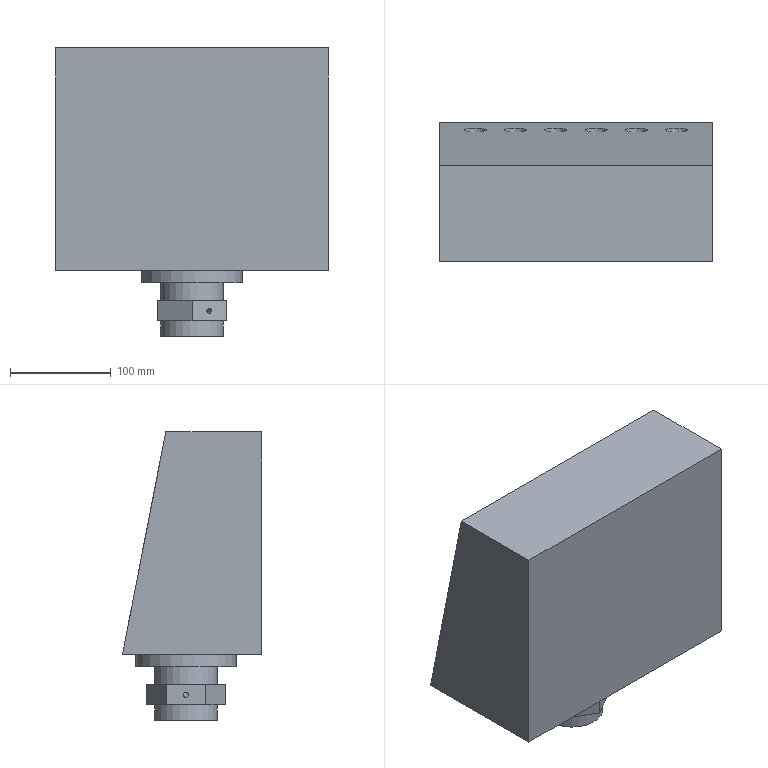Part | STEP file | 2_id534_x_t | 1 solid | 52 faces | box 270 x 138 x 285.853 mm | volume 7043394 mm3 | plane 31 | cylinder 15 | other 6 | commonest cylinder face diameters 6.5 x4 11 x4 5 x3 62 x2 48 x1 100 x1
STEP:
#1=CARTESIAN_POINT('',(1612.983,-177.049,402.));
#2=VERTEX_POINT('',#1);
#3=CARTESIAN_POINT('',(1620.,-200.,402.));
#4=DIRECTION('',(0.,0.,1.));
#5=DIRECTION('',(-0.2924,0.9563,0.));
#6=AXIS2_PLACEMENT_3D('',#3,#4,#5);
#7=CIRCLE('',#6,24.);
#8=EDGE_CURVE('',#2,#2,#7,.T.);
#9=ORIENTED_EDGE('',*,*,#8,.T.);
#10=EDGE_LOOP('',(#9));
#11=FACE_BOUND('',#10,.T.);
#12=CARTESIAN_POINT('',(1612.983,-222.951,337.));
#13=VERTEX_POINT('',#12);
#14=CARTESIAN_POINT('',(1620.,-200.,337.));
#15=DIRECTION('',(0.,0.,-1.));
#16=DIRECTION('',(-0.2924,-0.9563,0.));
#17=AXIS2_PLACEMENT_3D('',#14,#15,#16);
#18=CIRCLE('',#17,24.);
#19=EDGE_CURVE('',#13,#13,#18,.T.);
#20=ORIENTED_EDGE('',*,*,#19,.T.);
#21=EDGE_LOOP('',(#20));
#22=FACE_BOUND('',#21,.T.);
#23=CARTESIAN_POINT('',(1596.119,-197.609,361.269));
#24=VERTEX_POINT('',#23);
#25=CARTESIAN_POINT('',(1596.119,-197.609,361.269));
#26=CARTESIAN_POINT('',(1596.111,-197.691,361.001));
#27=CARTESIAN_POINT('',(1596.099,-197.82,360.744));
#28=CARTESIAN_POINT('',(1596.085,-197.986,360.519));
#29=CARTESIAN_POINT('',(1596.071,-198.152,360.294));
#30=CARTESIAN_POINT('',(1596.055,-198.358,360.094));
#31=CARTESIAN_POINT('',(1596.041,-198.589,359.936));
#32=CARTESIAN_POINT('',(1596.028,-198.821,359.778));
#33=CARTESIAN_POINT('',(1596.016,-199.083,359.658));
#34=CARTESIAN_POINT('',(1596.009,-199.354,359.585));
#35=CARTESIAN_POINT('',(1596.001,-199.624,359.513));
#36=CARTESIAN_POINT('',(1595.999,-199.91,359.486));
#37=CARTESIAN_POINT('',(1596.001,-200.189,359.507));
#38=CARTESIAN_POINT('',(1596.003,-200.466,359.528));
#39=CARTESIAN_POINT('',(1596.01,-200.744,359.597));
#40=CARTESIAN_POINT('',(1596.021,-200.999,359.708));
#41=CARTESIAN_POINT('',(1596.031,-201.255,359.82));
#42=CARTESIAN_POINT('',(1596.046,-201.494,359.976));
#43=CARTESIAN_POINT('',(1596.06,-201.699,360.166));
#44=CARTESIAN_POINT('',(1596.075,-201.904,360.356));
#45=CARTESIAN_POINT('',(1596.09,-202.079,360.584));
#46=CARTESIAN_POINT('',(1596.102,-202.21,360.831));
#47=CARTESIAN_POINT('',(1596.114,-202.341,361.079));
#48=CARTESIAN_POINT('',(1596.123,-202.431,361.353));
#49=CARTESIAN_POINT('',(1596.128,-202.472,361.63));
#50=CARTESIAN_POINT('',(1596.13,-202.491,361.752));
#51=CARTESIAN_POINT('',(1596.131,-202.5,361.876));
#52=CARTESIAN_POINT('',(1596.131,-202.5,362.));
#53=CARTESIAN_POINT('',(1596.131,-202.5,362.246));
#54=CARTESIAN_POINT('',(1596.127,-202.463,362.495));
#55=CARTESIAN_POINT('',(1596.119,-202.391,362.731));
#56=CARTESIAN_POINT('',(1596.111,-202.309,362.999));
#57=CARTESIAN_POINT('',(1596.099,-202.18,363.256));
#58=CARTESIAN_POINT('',(1596.085,-202.014,363.481));
#59=CARTESIAN_POINT('',(1596.071,-201.848,363.706));
#60=CARTESIAN_POINT('',(1596.055,-201.642,363.906));
#61=CARTESIAN_POINT('',(1596.041,-201.411,364.064));
#62=CARTESIAN_POINT('',(1596.028,-201.179,364.222));
#63=CARTESIAN_POINT('',(1596.016,-200.917,364.342));
#64=CARTESIAN_POINT('',(1596.009,-200.646,364.415));
#65=CARTESIAN_POINT('',(1596.001,-200.376,364.487));
#66=CARTESIAN_POINT('',(1595.999,-200.09,364.514));
#67=CARTESIAN_POINT('',(1596.001,-199.811,364.493));
#68=CARTESIAN_POINT('',(1596.003,-199.534,364.472));
#69=CARTESIAN_POINT('',(1596.01,-199.256,364.403));
#70=CARTESIAN_POINT('',(1596.021,-199.001,364.292));
#71=CARTESIAN_POINT('',(1596.031,-198.745,364.18));
#72=CARTESIAN_POINT('',(1596.046,-198.506,364.024));
#73=CARTESIAN_POINT('',(1596.06,-198.301,363.834));
#74=CARTESIAN_POINT('',(1596.075,-198.096,363.644));
#75=CARTESIAN_POINT('',(1596.09,-197.921,363.416));
#76=CARTESIAN_POINT('',(1596.102,-197.79,363.169));
#77=CARTESIAN_POINT('',(1596.114,-197.659,362.921));
#78=CARTESIAN_POINT('',(1596.123,-197.569,362.647));
#79=CARTESIAN_POINT('',(1596.128,-197.528,362.37));
#80=CARTESIAN_POINT('',(1596.132,-197.486,362.094));
#81=CARTESIAN_POINT('',(1596.131,-197.492,361.807));
#82=CARTESIAN_POINT('',(1596.126,-197.544,361.533));
#83=CARTESIAN_POINT('',(1596.124,-197.561,361.444));
#84=CARTESIAN_POINT('',(1596.122,-197.583,361.356));
#85=CARTESIAN_POINT('',(1596.119,-197.609,361.269));
#86=B_SPLINE_CURVE_WITH_KNOTS('',3,(#25,#26,#27,#28,#29,#30,#31,#32,#33,#34,#35,#36,#37,#38,#39,#40,#41,#42,#43,#44,#45,#46,#47,#48,#49,#50,#51,#52,#53,#54,#55,#56,#57,#58,#59,#60,#61,#62,#63,#64,#65,#66,#67,#68,#69,#70,#71,#72,#73,#74,#75,#76,#77,#78,#79,#80,#81,#82,#83,#84,#85),.UNSPECIFIED.,.T.,.F.,(1,3,3,3,3,3,3,3,3,3,3,3,3,3,3,3,3,3,3,3,3,3,1),(-0.01715,0.,0.05373,0.1074,0.1613,0.2149,0.2683,0.3218,0.3756,0.4294,0.4528,0.4999,0.5537,0.6074,0.6612,0.7149,0.7683,0.8218,0.8755,0.9293,0.9829,1.,1.054),.UNSPECIFIED.);
#87=EDGE_CURVE('',#24,#24,#86,.T.);
#88=ORIENTED_EDGE('',*,*,#87,.T.);
#89=EDGE_LOOP('',(#88));
#90=FACE_BOUND('',#89,.T.);
#91=CARTESIAN_POINT('',(1629.77,-178.078,362.));
#92=VERTEX_POINT('',#91);
#93=CARTESIAN_POINT('',(1629.77,-178.078,362.));
#94=CARTESIAN_POINT('',(1629.77,-178.078,362.279));
#95=CARTESIAN_POINT('',(1629.814,-178.098,362.562));
#96=CARTESIAN_POINT('',(1629.898,-178.136,362.825));
#97=CARTESIAN_POINT('',(1629.982,-178.174,363.088));
#98=CARTESIAN_POINT('',(1630.109,-178.232,363.339));
#99=CARTESIAN_POINT('',(1630.266,-178.307,363.557));
#100=CARTESIAN_POINT('',(1630.424,-178.381,363.776));
#101=CARTESIAN_POINT('',(1630.617,-178.475,363.967));
#102=CARTESIAN_POINT('',(1630.829,-178.582,364.116));
#103=CARTESIAN_POINT('',(1631.041,-178.689,364.265));
#104=CARTESIAN_POINT('',(1631.277,-178.813,364.376));
#105=CARTESIAN_POINT('',(1631.517,-178.944,364.438));
#106=CARTESIAN_POINT('',(1631.756,-179.075,364.5));
#107=CARTESIAN_POINT('',(1632.005,-179.217,364.516));
#108=CARTESIAN_POINT('',(1632.244,-179.358,364.484));
#109=CARTESIAN_POINT('',(1632.375,-179.436,364.467));
#110=CARTESIAN_POINT('',(1632.503,-179.514,364.435));
#111=CARTESIAN_POINT('',(1632.627,-179.59,364.391));
#112=CARTESIAN_POINT('',(1632.855,-179.731,364.309));
#113=CARTESIAN_POINT('',(1633.072,-179.871,364.18));
#114=CARTESIAN_POINT('',(1633.26,-179.996,364.014));
#115=CARTESIAN_POINT('',(1633.448,-180.12,363.848));
#116=CARTESIAN_POINT('',(1633.613,-180.234,363.642));
#117=CARTESIAN_POINT('',(1633.743,-180.324,363.411));
#118=CARTESIAN_POINT('',(1633.873,-180.415,363.179));
#119=CARTESIAN_POINT('',(1633.971,-180.486,362.917));
#120=CARTESIAN_POINT('',(1634.031,-180.528,362.647));
#121=CARTESIAN_POINT('',(1634.089,-180.571,362.376));
#122=CARTESIAN_POINT('',(1634.111,-180.587,362.09));
#123=CARTESIAN_POINT('',(1634.094,-180.574,361.811));
#124=CARTESIAN_POINT('',(1634.077,-180.562,361.534));
#125=CARTESIAN_POINT('',(1634.021,-180.521,361.256));
#126=CARTESIAN_POINT('',(1633.93,-180.456,361.001));
#127=CARTESIAN_POINT('',(1633.839,-180.391,360.745));
#128=CARTESIAN_POINT('',(1633.71,-180.301,360.506));
#129=CARTESIAN_POINT('',(1633.554,-180.193,360.301));
#130=CARTESIAN_POINT('',(1633.396,-180.086,360.096));
#131=CARTESIAN_POINT('',(1633.206,-179.959,359.921));
#132=CARTESIAN_POINT('',(1632.998,-179.824,359.79));
#133=CARTESIAN_POINT('',(1632.79,-179.69,359.659));
#134=CARTESIAN_POINT('',(1632.557,-179.545,359.569));
#135=CARTESIAN_POINT('',(1632.319,-179.403,359.528));
#136=CARTESIAN_POINT('',(1632.082,-179.261,359.486));
#137=CARTESIAN_POINT('',(1631.833,-179.118,359.492));
#138=CARTESIAN_POINT('',(1631.593,-178.986,359.544));
#139=CARTESIAN_POINT('',(1631.354,-178.854,359.596));
#140=CARTESIAN_POINT('',(1631.116,-178.728,359.696));
#141=CARTESIAN_POINT('',(1630.901,-178.619,359.835));
#142=CARTESIAN_POINT('',(1630.83,-178.582,359.881));
#143=CARTESIAN_POINT('',(1630.761,-178.548,359.931));
#144=CARTESIAN_POINT('',(1630.694,-178.514,359.986));
#145=CARTESIAN_POINT('',(1630.492,-178.414,360.152));
#146=CARTESIAN_POINT('',(1630.312,-178.328,360.358));
#147=CARTESIAN_POINT('',(1630.168,-178.26,360.589));
#148=CARTESIAN_POINT('',(1630.024,-178.193,360.821));
#149=CARTESIAN_POINT('',(1629.914,-178.143,361.083));
#150=CARTESIAN_POINT('',(1629.848,-178.113,361.353));
#151=CARTESIAN_POINT('',(1629.796,-178.09,361.563));
#152=CARTESIAN_POINT('',(1629.77,-178.078,361.783));
#153=CARTESIAN_POINT('',(1629.77,-178.078,362.));
#154=B_SPLINE_CURVE_WITH_KNOTS('',3,(#93,#94,#95,#96,#97,#98,#99,#100,#101,#102,#103,#104,#105,#106,#107,#108,#109,#110,#111,#112,#113,#114,#115,#116,#117,#118,#119,#120,#121,#122,#123,#124,#125,#126,#127,#128,#129,#130,#131,#132,#133,#134,#135,#136,#137,#138,#139,#140,#141,#142,#143,#144,#145,#146,#147,#148,#149,#150,#151,#152,#153),.UNSPECIFIED.,.T.,.F.,(1,3,3,3,3,3,3,3,3,3,3,3,3,3,3,3,3,3,3,3,3,3,1),(-0.04147,0.,0.05352,0.107,0.1607,0.2146,0.2682,0.2972,0.3509,0.4046,0.4584,0.5121,0.5655,0.619,0.6727,0.7265,0.7801,0.8335,0.851,0.9047,0.9585,1.,1.054),.UNSPECIFIED.);
#155=EDGE_CURVE('',#92,#92,#154,.T.);
#156=ORIENTED_EDGE('',*,*,#155,.T.);
#157=EDGE_LOOP('',(#156));
#158=FACE_BOUND('',#157,.T.);
#159=CARTESIAN_POINT('',(1632.627,-220.41,359.609));
#160=VERTEX_POINT('',#159);
#161=CARTESIAN_POINT('',(1632.627,-220.41,359.609));
#162=CARTESIAN_POINT('',(1632.855,-220.269,359.691));
#163=CARTESIAN_POINT('',(1633.072,-220.129,359.82));
#164=CARTESIAN_POINT('',(1633.26,-220.004,359.986));
#165=CARTESIAN_POINT('',(1633.448,-219.88,360.152));
#166=CARTESIAN_POINT('',(1633.613,-219.766,360.358));
#167=CARTESIAN_POINT('',(1633.743,-219.676,360.589));
#168=CARTESIAN_POINT('',(1633.873,-219.585,360.821));
#169=CARTESIAN_POINT('',(1633.971,-219.514,361.083));
#170=CARTESIAN_POINT('',(1634.031,-219.472,361.353));
#171=CARTESIAN_POINT('',(1634.076,-219.439,361.563));
#172=CARTESIAN_POINT('',(1634.1,-219.422,361.783));
#173=CARTESIAN_POINT('',(1634.1,-219.422,362.));
#174=CARTESIAN_POINT('',(1634.1,-219.422,362.279));
#175=CARTESIAN_POINT('',(1634.061,-219.45,362.562));
#176=CARTESIAN_POINT('',(1633.986,-219.504,362.825));
#177=CARTESIAN_POINT('',(1633.911,-219.558,363.088));
#178=CARTESIAN_POINT('',(1633.797,-219.638,363.339));
#179=CARTESIAN_POINT('',(1633.654,-219.737,363.557));
#180=CARTESIAN_POINT('',(1633.51,-219.837,363.776));
#181=CARTESIAN_POINT('',(1633.333,-219.957,363.967));
#182=CARTESIAN_POINT('',(1633.134,-220.087,364.116));
#183=CARTESIAN_POINT('',(1632.936,-220.217,364.265));
#184=CARTESIAN_POINT('',(1632.71,-220.36,364.376));
#185=CARTESIAN_POINT('',(1632.477,-220.502,364.438));
#186=CARTESIAN_POINT('',(1632.244,-220.644,364.5));
#187=CARTESIAN_POINT('',(1631.996,-220.789,364.516));
#188=CARTESIAN_POINT('',(1631.754,-220.925,364.484));
#189=CARTESIAN_POINT('',(1631.513,-221.06,364.452));
#190=CARTESIAN_POINT('',(1631.271,-221.19,364.373));
#191=CARTESIAN_POINT('',(1631.048,-221.306,364.252));
#192=CARTESIAN_POINT('',(1630.925,-221.37,364.185));
#193=CARTESIAN_POINT('',(1630.806,-221.43,364.105));
#194=CARTESIAN_POINT('',(1630.694,-221.486,364.014));
#195=CARTESIAN_POINT('',(1630.492,-221.586,363.848));
#196=CARTESIAN_POINT('',(1630.312,-221.672,363.642));
#197=CARTESIAN_POINT('',(1630.168,-221.74,363.411));
#198=CARTESIAN_POINT('',(1630.024,-221.807,363.179));
#199=CARTESIAN_POINT('',(1629.914,-221.857,362.917));
#200=CARTESIAN_POINT('',(1629.848,-221.887,362.647));
#201=CARTESIAN_POINT('',(1629.781,-221.916,362.376));
#202=CARTESIAN_POINT('',(1629.757,-221.927,362.09));
#203=CARTESIAN_POINT('',(1629.776,-221.919,361.811));
#204=CARTESIAN_POINT('',(1629.796,-221.91,361.534));
#205=CARTESIAN_POINT('',(1629.859,-221.882,361.256));
#206=CARTESIAN_POINT('',(1629.961,-221.835,361.001));
#207=CARTESIAN_POINT('',(1630.062,-221.789,360.745));
#208=CARTESIAN_POINT('',(1630.205,-221.723,360.506));
#209=CARTESIAN_POINT('',(1630.376,-221.641,360.301));
#210=CARTESIAN_POINT('',(1630.548,-221.559,360.096));
#211=CARTESIAN_POINT('',(1630.753,-221.458,359.921));
#212=CARTESIAN_POINT('',(1630.974,-221.344,359.79));
#213=CARTESIAN_POINT('',(1631.194,-221.231,359.659));
#214=CARTESIAN_POINT('',(1631.436,-221.102,359.569));
#215=CARTESIAN_POINT('',(1631.678,-220.967,359.528));
#216=CARTESIAN_POINT('',(1631.919,-220.833,359.486));
#217=CARTESIAN_POINT('',(1632.168,-220.689,359.492));
#218=CARTESIAN_POINT('',(1632.402,-220.547,359.544));
#219=CARTESIAN_POINT('',(1632.479,-220.501,359.561));
#220=CARTESIAN_POINT('',(1632.554,-220.455,359.583));
#221=CARTESIAN_POINT('',(1632.627,-220.41,359.609));
#222=B_SPLINE_CURVE_WITH_KNOTS('',3,(#161,#162,#163,#164,#165,#166,#167,#168,#169,#170,#171,#172,#173,#174,#175,#176,#177,#178,#179,#180,#181,#182,#183,#184,#185,#186,#187,#188,#189,#190,#191,#192,#193,#194,#195,#196,#197,#198,#199,#200,#201,#202,#203,#204,#205,#206,#207,#208,#209,#210,#211,#212,#213,#214,#215,#216,#217,#218,#219,#220,#221),.UNSPECIFIED.,.T.,.F.,(1,3,3,3,3,3,3,3,3,3,3,3,3,3,3,3,3,3,3,3,3,3,1),(-0.01715,0.,0.05373,0.1075,0.1613,0.2028,0.2563,0.3098,0.3635,0.4173,0.4709,0.5243,0.5536,0.6074,0.6612,0.7148,0.7683,0.8217,0.8755,0.9293,0.9828,1.,1.054),.UNSPECIFIED.);
#223=EDGE_CURVE('',#160,#160,#222,.T.);
#224=ORIENTED_EDGE('',*,*,#223,.T.);
#225=EDGE_LOOP('',(#224));
#226=FACE_BOUND('',#225,.T.);
#227=CARTESIAN_POINT('',(1620.,-200.,402.));
#228=DIRECTION('',(0.,0.,-1.));
#229=DIRECTION('',(0.2924,-0.9563,0.));
#230=AXIS2_PLACEMENT_3D('',#227,#228,#229);
#231=CYLINDRICAL_SURFACE('',#230,24.);
#232=ADVANCED_FACE('',(#11,#22,#90,#158,#226),#231,.F.);
#233=CARTESIAN_POINT('',(1605.381,-152.185,402.));
#234=VERTEX_POINT('',#233);
#235=CARTESIAN_POINT('',(1620.,-200.,402.));
#236=DIRECTION('',(0.,0.,1.));
#237=DIRECTION('',(-0.2924,0.9563,0.));
#238=AXIS2_PLACEMENT_3D('',#235,#236,#237);
#239=CIRCLE('',#238,50.);
#240=EDGE_CURVE('',#234,#234,#239,.T.);
#241=ORIENTED_EDGE('',*,*,#240,.F.);
#242=EDGE_LOOP('',(#241));
#243=FACE_BOUND('',#242,.T.);
#244=CARTESIAN_POINT('',(1605.381,-152.185,390.));
#245=VERTEX_POINT('',#244);
#246=CARTESIAN_POINT('',(1620.,-200.,390.));
#247=DIRECTION('',(0.,0.,1.));
#248=DIRECTION('',(-0.2924,0.9563,0.));
#249=AXIS2_PLACEMENT_3D('',#246,#247,#248);
#250=CIRCLE('',#249,50.);
#251=EDGE_CURVE('',#245,#245,#250,.T.);
#252=ORIENTED_EDGE('',*,*,#251,.T.);
#253=EDGE_LOOP('',(#252));
#254=FACE_BOUND('',#253,.T.);
#255=CARTESIAN_POINT('',(1620.,-200.,402.));
#256=DIRECTION('',(0.,0.,-1.));
#257=DIRECTION('',(0.2924,-0.9563,0.));
#258=AXIS2_PLACEMENT_3D('',#255,#256,#257);
#259=CYLINDRICAL_SURFACE('',#258,50.);
#260=ADVANCED_FACE('',(#243,#254),#259,.T.);
#261=CARTESIAN_POINT('',(1610.936,-229.645,352.));
#262=VERTEX_POINT('',#261);
#263=CARTESIAN_POINT('',(1620.,-200.,352.));
#264=DIRECTION('',(0.,0.,-1.));
#265=DIRECTION('',(-0.2924,-0.9563,0.));
#266=AXIS2_PLACEMENT_3D('',#263,#264,#265);
#267=CIRCLE('',#266,31.);
#268=EDGE_CURVE('',#262,#262,#267,.T.);
#269=ORIENTED_EDGE('',*,*,#268,.T.);
#270=EDGE_LOOP('',(#269));
#271=FACE_BOUND('',#270,.T.);
#272=CARTESIAN_POINT('',(1610.936,-229.645,337.));
#273=VERTEX_POINT('',#272);
#274=CARTESIAN_POINT('',(1620.,-200.,337.));
#275=DIRECTION('',(0.,0.,1.));
#276=DIRECTION('',(-0.2924,-0.9563,0.));
#277=AXIS2_PLACEMENT_3D('',#274,#275,#276);
#278=CIRCLE('',#277,31.);
#279=EDGE_CURVE('',#273,#273,#278,.T.);
#280=ORIENTED_EDGE('',*,*,#279,.T.);
#281=EDGE_LOOP('',(#280));
#282=FACE_BOUND('',#281,.T.);
#283=CARTESIAN_POINT('',(1620.,-200.,390.));
#284=DIRECTION('',(0.,0.,-1.));
#285=DIRECTION('',(0.2924,0.9563,0.));
#286=AXIS2_PLACEMENT_3D('',#283,#284,#285);
#287=CYLINDRICAL_SURFACE('',#286,31.);
#288=ADVANCED_FACE('',(#271,#282),#287,.T.);
#289=CARTESIAN_POINT('',(1610.936,-229.645,390.));
#290=VERTEX_POINT('',#289);
#291=CARTESIAN_POINT('',(1620.,-200.,390.));
#292=DIRECTION('',(0.,0.,1.));
#293=DIRECTION('',(-0.2924,-0.9563,0.));
#294=AXIS2_PLACEMENT_3D('',#291,#292,#293);
#295=CIRCLE('',#294,31.);
#296=EDGE_CURVE('',#290,#290,#295,.T.);
#297=ORIENTED_EDGE('',*,*,#296,.F.);
#298=EDGE_LOOP('',(#297));
#299=FACE_BOUND('',#298,.T.);
#300=CARTESIAN_POINT('',(1610.936,-229.645,372.));
#301=VERTEX_POINT('',#300);
#302=CARTESIAN_POINT('',(1620.,-200.,372.));
#303=DIRECTION('',(0.,0.,1.));
#304=DIRECTION('',(-0.2924,-0.9563,0.));
#305=AXIS2_PLACEMENT_3D('',#302,#303,#304);
#306=CIRCLE('',#305,31.);
#307=EDGE_CURVE('',#301,#301,#306,.T.);
#308=ORIENTED_EDGE('',*,*,#307,.T.);
#309=EDGE_LOOP('',(#308));
#310=FACE_BOUND('',#309,.T.);
#311=CARTESIAN_POINT('',(1620.,-200.,390.));
#312=DIRECTION('',(0.,0.,-1.));
#313=DIRECTION('',(0.2924,0.9563,0.));
#314=AXIS2_PLACEMENT_3D('',#311,#312,#313);
#315=CYLINDRICAL_SURFACE('',#314,31.);
#316=ADVANCED_FACE('',(#299,#310),#315,.T.);
#317=ORIENTED_EDGE('',*,*,#223,.F.);
#318=EDGE_LOOP('',(#317));
#319=FACE_BOUND('',#318,.T.);
#320=CARTESIAN_POINT('',(1636.367,-229.81,364.391));
#321=VERTEX_POINT('',#320);
#322=CARTESIAN_POINT('',(1637.,-229.445,362.));
#323=DIRECTION('',(-0.5,0.866,0.));
#324=DIRECTION('',(-0.2532,-0.1462,0.9563));
#325=AXIS2_PLACEMENT_3D('',#322,#323,#324);
#326=CIRCLE('',#325,2.5);
#327=EDGE_CURVE('',#321,#321,#326,.T.);
#328=ORIENTED_EDGE('',*,*,#327,.F.);
#329=EDGE_LOOP('',(#328));
#330=FACE_BOUND('',#329,.T.);
#331=CARTESIAN_POINT('',(1634.42,-224.976,362.));
#332=DIRECTION('',(-0.5,0.866,0.));
#333=DIRECTION('',(0.2532,0.1462,-0.9563));
#334=AXIS2_PLACEMENT_3D('',#331,#332,#333);
#335=CYLINDRICAL_SURFACE('',#334,2.5);
#336=ADVANCED_FACE('',(#319,#330),#335,.F.);
#337=ORIENTED_EDGE('',*,*,#155,.F.);
#338=EDGE_LOOP('',(#337));
#339=FACE_BOUND('',#338,.T.);
#340=CARTESIAN_POINT('',(1636.367,-170.19,359.609));
#341=VERTEX_POINT('',#340);
#342=CARTESIAN_POINT('',(1637.,-170.555,362.));
#343=DIRECTION('',(-0.5,-0.866,0.));
#344=DIRECTION('',(-0.2532,0.1462,-0.9563));
#345=AXIS2_PLACEMENT_3D('',#342,#343,#344);
#346=CIRCLE('',#345,2.5);
#347=EDGE_CURVE('',#341,#341,#346,.T.);
#348=ORIENTED_EDGE('',*,*,#347,.F.);
#349=EDGE_LOOP('',(#348));
#350=FACE_BOUND('',#349,.T.);
#351=CARTESIAN_POINT('',(1634.42,-175.024,362.));
#352=DIRECTION('',(-0.5,-0.866,0.));
#353=DIRECTION('',(0.2532,-0.1462,0.9563));
#354=AXIS2_PLACEMENT_3D('',#351,#352,#353);
#355=CYLINDRICAL_SURFACE('',#354,2.5);
#356=ADVANCED_FACE('',(#339,#350),#355,.F.);
#357=ORIENTED_EDGE('',*,*,#87,.F.);
#358=EDGE_LOOP('',(#357));
#359=FACE_BOUND('',#358,.T.);
#360=CARTESIAN_POINT('',(1586.,-202.391,362.731));
#361=VERTEX_POINT('',#360);
#362=CARTESIAN_POINT('',(1586.,-200.,362.));
#363=DIRECTION('',(1.,0.,0.));
#364=DIRECTION('',(0.,-0.9563,0.2924));
#365=AXIS2_PLACEMENT_3D('',#362,#363,#364);
#366=CIRCLE('',#365,2.5);
#367=EDGE_CURVE('',#361,#361,#366,.T.);
#368=ORIENTED_EDGE('',*,*,#367,.F.);
#369=EDGE_LOOP('',(#368));
#370=FACE_BOUND('',#369,.T.);
#371=CARTESIAN_POINT('',(1586.,-200.,362.));
#372=DIRECTION('',(1.,0.,0.));
#373=DIRECTION('',(0.,0.9563,-0.2924));
#374=AXIS2_PLACEMENT_3D('',#371,#372,#373);
#375=CYLINDRICAL_SURFACE('',#374,2.5);
#376=ADVANCED_FACE('',(#359,#370),#375,.F.);
#377=CARTESIAN_POINT('',(1579.05,-203.108,402.));
#378=VERTEX_POINT('',#377);
#379=CARTESIAN_POINT('',(1580.,-200.,402.));
#380=DIRECTION('',(0.,0.,-1.));
#381=DIRECTION('',(-0.2924,-0.9563,0.));
#382=AXIS2_PLACEMENT_3D('',#379,#380,#381);
#383=CIRCLE('',#382,3.25);
#384=EDGE_CURVE('',#378,#378,#383,.T.);
#385=ORIENTED_EDGE('',*,*,#384,.F.);
#386=EDGE_LOOP('',(#385));
#387=FACE_BOUND('',#386,.T.);
#388=CARTESIAN_POINT('',(1580.,-203.25,396.5));
#389=VERTEX_POINT('',#388);
#390=CARTESIAN_POINT('',(1580.,-200.,396.5));
#391=DIRECTION('',(0.,0.,-1.));
#392=DIRECTION('',(0.,-1.,0.));
#393=AXIS2_PLACEMENT_3D('',#390,#391,#392);
#394=CIRCLE('',#393,3.25);
#395=EDGE_CURVE('',#389,#389,#394,.T.);
#396=ORIENTED_EDGE('',*,*,#395,.T.);
#397=EDGE_LOOP('',(#396));
#398=FACE_BOUND('',#397,.T.);
#399=CARTESIAN_POINT('',(1580.,-200.,390.));
#400=DIRECTION('',(0.,0.,1.));
#401=DIRECTION('',(0.2924,0.9563,0.));
#402=AXIS2_PLACEMENT_3D('',#399,#400,#401);
#403=CYLINDRICAL_SURFACE('',#402,3.25);
#404=ADVANCED_FACE('',(#387,#398),#403,.F.);
#405=CARTESIAN_POINT('',(1580.,-205.5,396.5));
#406=VERTEX_POINT('',#405);
#407=CARTESIAN_POINT('',(1580.,-200.,396.5));
#408=DIRECTION('',(0.,0.,-1.));
#409=DIRECTION('',(0.,-1.,0.));
#410=AXIS2_PLACEMENT_3D('',#407,#408,#409);
#411=CIRCLE('',#410,5.5);
#412=EDGE_CURVE('',#406,#406,#411,.T.);
#413=ORIENTED_EDGE('',*,*,#412,.F.);
#414=EDGE_LOOP('',(#413));
#415=FACE_BOUND('',#414,.T.);
#416=CARTESIAN_POINT('',(1578.392,-205.26,390.));
#417=VERTEX_POINT('',#416);
#418=CARTESIAN_POINT('',(1580.,-200.,390.));
#419=DIRECTION('',(0.,0.,1.));
#420=DIRECTION('',(-0.2924,-0.9563,0.));
#421=AXIS2_PLACEMENT_3D('',#418,#419,#420);
#422=CIRCLE('',#421,5.5);
#423=EDGE_CURVE('',#417,#417,#422,.T.);
#424=ORIENTED_EDGE('',*,*,#423,.F.);
#425=EDGE_LOOP('',(#424));
#426=FACE_BOUND('',#425,.T.);
#427=CARTESIAN_POINT('',(1580.,-200.,390.));
#428=DIRECTION('',(0.,0.,1.));
#429=DIRECTION('',(0.2924,0.9563,0.));
#430=AXIS2_PLACEMENT_3D('',#427,#428,#429);
#431=CYLINDRICAL_SURFACE('',#430,5.5);
#432=ADVANCED_FACE('',(#415,#426),#431,.F.);
#433=CARTESIAN_POINT('',(1616.892,-159.05,402.));
#434=VERTEX_POINT('',#433);
#435=CARTESIAN_POINT('',(1620.,-160.,402.));
#436=DIRECTION('',(0.,0.,-1.));
#437=DIRECTION('',(-0.9563,0.2924,0.));
#438=AXIS2_PLACEMENT_3D('',#435,#436,#437);
#439=CIRCLE('',#438,3.25);
#440=EDGE_CURVE('',#434,#434,#439,.T.);
#441=ORIENTED_EDGE('',*,*,#440,.F.);
#442=EDGE_LOOP('',(#441));
#443=FACE_BOUND('',#442,.T.);
#444=CARTESIAN_POINT('',(1620.,-163.25,396.5));
#445=VERTEX_POINT('',#444);
#446=CARTESIAN_POINT('',(1620.,-160.,396.5));
#447=DIRECTION('',(0.,0.,-1.));
#448=DIRECTION('',(0.,-1.,0.));
#449=AXIS2_PLACEMENT_3D('',#446,#447,#448);
#450=CIRCLE('',#449,3.25);
#451=EDGE_CURVE('',#445,#445,#450,.T.);
#452=ORIENTED_EDGE('',*,*,#451,.T.);
#453=EDGE_LOOP('',(#452));
#454=FACE_BOUND('',#453,.T.);
#455=CARTESIAN_POINT('',(1620.,-160.,390.));
#456=DIRECTION('',(0.,0.,1.));
#457=DIRECTION('',(0.9563,-0.2924,0.));
#458=AXIS2_PLACEMENT_3D('',#455,#456,#457);
#459=CYLINDRICAL_SURFACE('',#458,3.25);
#460=ADVANCED_FACE('',(#443,#454),#459,.F.);
#461=CARTESIAN_POINT('',(1660.95,-196.892,402.));
#462=VERTEX_POINT('',#461);
#463=CARTESIAN_POINT('',(1660.,-200.,402.));
#464=DIRECTION('',(0.,0.,-1.));
#465=DIRECTION('',(0.2924,0.9563,0.));
#466=AXIS2_PLACEMENT_3D('',#463,#464,#465);
#467=CIRCLE('',#466,3.25);
#468=EDGE_CURVE('',#462,#462,#467,.T.);
#469=ORIENTED_EDGE('',*,*,#468,.F.);
#470=EDGE_LOOP('',(#469));
#471=FACE_BOUND('',#470,.T.);
#472=CARTESIAN_POINT('',(1660.,-203.25,396.5));
#473=VERTEX_POINT('',#472);
#474=CARTESIAN_POINT('',(1660.,-200.,396.5));
#475=DIRECTION('',(0.,0.,-1.));
#476=DIRECTION('',(0.,-1.,0.));
#477=AXIS2_PLACEMENT_3D('',#474,#475,#476);
#478=CIRCLE('',#477,3.25);
#479=EDGE_CURVE('',#473,#473,#478,.T.);
#480=ORIENTED_EDGE('',*,*,#479,.T.);
#481=EDGE_LOOP('',(#480));
#482=FACE_BOUND('',#481,.T.);
#483=CARTESIAN_POINT('',(1660.,-200.,390.));
#484=DIRECTION('',(0.,0.,1.));
#485=DIRECTION('',(-0.2924,-0.9563,0.));
#486=AXIS2_PLACEMENT_3D('',#483,#484,#485);
#487=CYLINDRICAL_SURFACE('',#486,3.25);
#488=ADVANCED_FACE('',(#471,#482),#487,.F.);
#489=CARTESIAN_POINT('',(1623.108,-240.95,402.));
#490=VERTEX_POINT('',#489);
#491=CARTESIAN_POINT('',(1620.,-240.,402.));
#492=DIRECTION('',(0.,0.,-1.));
#493=DIRECTION('',(0.9563,-0.2924,0.));
#494=AXIS2_PLACEMENT_3D('',#491,#492,#493);
#495=CIRCLE('',#494,3.25);
#496=EDGE_CURVE('',#490,#490,#495,.T.);
#497=ORIENTED_EDGE('',*,*,#496,.F.);
#498=EDGE_LOOP('',(#497));
#499=FACE_BOUND('',#498,.T.);
#500=CARTESIAN_POINT('',(1623.108,-240.95,396.5));
#501=VERTEX_POINT('',#500);
#502=CARTESIAN_POINT('',(1620.,-240.,396.5));
#503=DIRECTION('',(0.,0.,-1.));
#504=DIRECTION('',(0.9563,-0.2924,0.));
#505=AXIS2_PLACEMENT_3D('',#502,#503,#504);
#506=CIRCLE('',#505,3.25);
#507=EDGE_CURVE('',#501,#501,#506,.T.);
#508=ORIENTED_EDGE('',*,*,#507,.T.);
#509=EDGE_LOOP('',(#508));
#510=FACE_BOUND('',#509,.T.);
#511=CARTESIAN_POINT('',(1620.,-240.,390.));
#512=DIRECTION('',(0.,0.,1.));
#513=DIRECTION('',(-0.9563,0.2924,0.));
#514=AXIS2_PLACEMENT_3D('',#511,#512,#513);
#515=CYLINDRICAL_SURFACE('',#514,3.25);
#516=ADVANCED_FACE('',(#499,#510),#515,.F.);
#517=CARTESIAN_POINT('',(1620.,-165.5,396.5));
#518=VERTEX_POINT('',#517);
#519=CARTESIAN_POINT('',(1620.,-160.,396.5));
#520=DIRECTION('',(0.,0.,-1.));
#521=DIRECTION('',(0.,-1.,0.));
#522=AXIS2_PLACEMENT_3D('',#519,#520,#521);
#523=CIRCLE('',#522,5.5);
#524=EDGE_CURVE('',#518,#518,#523,.T.);
#525=ORIENTED_EDGE('',*,*,#524,.F.);
#526=EDGE_LOOP('',(#525));
#527=FACE_BOUND('',#526,.T.);
#528=CARTESIAN_POINT('',(1614.74,-158.392,390.));
#529=VERTEX_POINT('',#528);
#530=CARTESIAN_POINT('',(1620.,-160.,390.));
#531=DIRECTION('',(0.,0.,1.));
#532=DIRECTION('',(-0.9563,0.2924,0.));
#533=AXIS2_PLACEMENT_3D('',#530,#531,#532);
#534=CIRCLE('',#533,5.5);
#535=EDGE_CURVE('',#529,#529,#534,.T.);
#536=ORIENTED_EDGE('',*,*,#535,.F.);
#537=EDGE_LOOP('',(#536));
#538=FACE_BOUND('',#537,.T.);
#539=CARTESIAN_POINT('',(1620.,-160.,390.));
#540=DIRECTION('',(0.,0.,1.));
#541=DIRECTION('',(0.9563,-0.2924,0.));
#542=AXIS2_PLACEMENT_3D('',#539,#540,#541);
#543=CYLINDRICAL_SURFACE('',#542,5.5);
#544=ADVANCED_FACE('',(#527,#538),#543,.F.);
#545=CARTESIAN_POINT('',(1660.,-205.5,396.5));
#546=VERTEX_POINT('',#545);
#547=CARTESIAN_POINT('',(1660.,-200.,396.5));
#548=DIRECTION('',(0.,0.,-1.));
#549=DIRECTION('',(0.,-1.,0.));
#550=AXIS2_PLACEMENT_3D('',#547,#548,#549);
#551=CIRCLE('',#550,5.5);
#552=EDGE_CURVE('',#546,#546,#551,.T.);
#553=ORIENTED_EDGE('',*,*,#552,.F.);
#554=EDGE_LOOP('',(#553));
#555=FACE_BOUND('',#554,.T.);
#556=CARTESIAN_POINT('',(1661.608,-194.74,390.));
#557=VERTEX_POINT('',#556);
#558=CARTESIAN_POINT('',(1660.,-200.,390.));
#559=DIRECTION('',(0.,0.,1.));
#560=DIRECTION('',(0.2924,0.9563,0.));
#561=AXIS2_PLACEMENT_3D('',#558,#559,#560);
#562=CIRCLE('',#561,5.5);
#563=EDGE_CURVE('',#557,#557,#562,.T.);
#564=ORIENTED_EDGE('',*,*,#563,.F.);
#565=EDGE_LOOP('',(#564));
#566=FACE_BOUND('',#565,.T.);
#567=CARTESIAN_POINT('',(1660.,-200.,390.));
#568=DIRECTION('',(0.,0.,1.));
#569=DIRECTION('',(-0.2924,-0.9563,0.));
#570=AXIS2_PLACEMENT_3D('',#567,#568,#569);
#571=CYLINDRICAL_SURFACE('',#570,5.5);
#572=ADVANCED_FACE('',(#555,#566),#571,.F.);
#573=CARTESIAN_POINT('',(1625.26,-241.608,396.5));
#574=VERTEX_POINT('',#573);
#575=CARTESIAN_POINT('',(1620.,-240.,396.5));
#576=DIRECTION('',(0.,0.,-1.));
#577=DIRECTION('',(0.9563,-0.2924,0.));
#578=AXIS2_PLACEMENT_3D('',#575,#576,#577);
#579=CIRCLE('',#578,5.5);
#580=EDGE_CURVE('',#574,#574,#579,.T.);
#581=ORIENTED_EDGE('',*,*,#580,.F.);
#582=EDGE_LOOP('',(#581));
#583=FACE_BOUND('',#582,.T.);
#584=CARTESIAN_POINT('',(1625.26,-241.608,390.));
#585=VERTEX_POINT('',#584);
#586=CARTESIAN_POINT('',(1620.,-240.,390.));
#587=DIRECTION('',(0.,0.,1.));
#588=DIRECTION('',(0.9563,-0.2924,0.));
#589=AXIS2_PLACEMENT_3D('',#586,#587,#588);
#590=CIRCLE('',#589,5.5);
#591=EDGE_CURVE('',#585,#585,#590,.T.);
#592=ORIENTED_EDGE('',*,*,#591,.F.);
#593=EDGE_LOOP('',(#592));
#594=FACE_BOUND('',#593,.T.);
#595=CARTESIAN_POINT('',(1620.,-240.,390.));
#596=DIRECTION('',(0.,0.,1.));
#597=DIRECTION('',(-0.9563,0.2924,0.));
#598=AXIS2_PLACEMENT_3D('',#595,#596,#597);
#599=CYLINDRICAL_SURFACE('',#598,5.5);
#600=ADVANCED_FACE('',(#583,#594),#599,.F.);
#601=CARTESIAN_POINT('',(1731.,-169.28,436.981));
#602=VERTEX_POINT('',#601);
#603=CARTESIAN_POINT('',(1720.,-169.28,436.981));
#604=DIRECTION('',(0.,0.9816,0.1911));
#605=DIRECTION('',(1.,0.,0.));
#606=AXIS2_PLACEMENT_3D('',#603,#604,#605);
#607=ELLIPSE('',#606,11.,10.797);
#608=EDGE_CURVE('',#602,#602,#607,.T.);
#609=ORIENTED_EDGE('',*,*,#608,.F.);
#610=EDGE_LOOP('',(#609));
#611=FACE_BOUND('',#610,.T.);
#612=CARTESIAN_POINT('',(1731.,-144.741,441.759));
#613=VERTEX_POINT('',#612);
#614=CARTESIAN_POINT('',(1720.,-144.741,441.759));
#615=DIRECTION('',(0.,-0.9816,-0.1911));
#616=DIRECTION('',(1.,0.,0.));
#617=AXIS2_PLACEMENT_3D('',#614,#615,#616);
#618=ELLIPSE('',#617,11.,10.797);
#619=EDGE_CURVE('',#613,#613,#618,.T.);
#620=ORIENTED_EDGE('',*,*,#619,.F.);
#621=EDGE_LOOP('',(#620));
#622=FACE_BOUND('',#621,.T.);
#623=CARTESIAN_POINT('',(1709.,-157.011,439.37));
#624=CARTESIAN_POINT('',(1709.,-154.947,428.772));
#625=CARTESIAN_POINT('',(1720.,-154.947,428.772));
#626=CARTESIAN_POINT('',(1731.,-154.947,428.772));
#627=CARTESIAN_POINT('',(1731.,-157.011,439.37));
#628=CARTESIAN_POINT('',(1731.,-159.074,449.968));
#629=CARTESIAN_POINT('',(1720.,-159.074,449.968));
#630=CARTESIAN_POINT('',(1709.,-159.074,449.968));
#631=CARTESIAN_POINT('',(1709.,-157.011,439.37));
#632=(BOUNDED_CURVE()B_SPLINE_CURVE(2,(#623,#624,#625,#626,#627,#628,#629,#630,#631),.UNSPECIFIED.,.T.,.F.)B_SPLINE_CURVE_WITH_KNOTS((1,2,2,2,2,2,1),(-0.25,0.,0.25,0.5,0.75,1.,1.25),.UNSPECIFIED.)CURVE()GEOMETRIC_REPRESENTATION_ITEM()RATIONAL_B_SPLINE_CURVE((1.,0.7071,1.,0.7071,1.,0.7071,1.,0.7071,1.))REPRESENTATION_ITEM(''));
#633=DIRECTION('',(0.,-0.9816,-0.1911));
#634=VECTOR('',#633,1.);
#635=SURFACE_OF_LINEAR_EXTRUSION('',#632,#634);
#636=ADVANCED_FACE('',(#611,#622),#635,.F.);
#637=CARTESIAN_POINT('',(1691.,-169.28,436.981));
#638=VERTEX_POINT('',#637);
#639=CARTESIAN_POINT('',(1680.,-169.28,436.981));
#640=DIRECTION('',(0.,0.9816,0.1911));
#641=DIRECTION('',(1.,0.,0.));
#642=AXIS2_PLACEMENT_3D('',#639,#640,#641);
#643=ELLIPSE('',#642,11.,10.797);
#644=EDGE_CURVE('',#638,#638,#643,.T.);
#645=ORIENTED_EDGE('',*,*,#644,.F.);
#646=EDGE_LOOP('',(#645));
#647=FACE_BOUND('',#646,.T.);
#648=CARTESIAN_POINT('',(1691.,-144.741,441.759));
#649=VERTEX_POINT('',#648);
#650=CARTESIAN_POINT('',(1680.,-144.741,441.759));
#651=DIRECTION('',(0.,-0.9816,-0.1911));
#652=DIRECTION('',(1.,0.,0.));
#653=AXIS2_PLACEMENT_3D('',#650,#651,#652);
#654=ELLIPSE('',#653,11.,10.797);
#655=EDGE_CURVE('',#649,#649,#654,.T.);
#656=ORIENTED_EDGE('',*,*,#655,.F.);
#657=EDGE_LOOP('',(#656));
#658=FACE_BOUND('',#657,.T.);
#659=CARTESIAN_POINT('',(1669.,-157.011,439.37));
#660=CARTESIAN_POINT('',(1669.,-154.947,428.772));
#661=CARTESIAN_POINT('',(1680.,-154.947,428.772));
#662=CARTESIAN_POINT('',(1691.,-154.947,428.772));
#663=CARTESIAN_POINT('',(1691.,-157.011,439.37));
#664=CARTESIAN_POINT('',(1691.,-159.074,449.968));
#665=CARTESIAN_POINT('',(1680.,-159.074,449.968));
#666=CARTESIAN_POINT('',(1669.,-159.074,449.968));
#667=CARTESIAN_POINT('',(1669.,-157.011,439.37));
#668=(BOUNDED_CURVE()B_SPLINE_CURVE(2,(#659,#660,#661,#662,#663,#664,#665,#666,#667),.UNSPECIFIED.,.T.,.F.)B_SPLINE_CURVE_WITH_KNOTS((1,2,2,2,2,2,1),(-0.25,0.,0.25,0.5,0.75,1.,1.25),.UNSPECIFIED.)CURVE()GEOMETRIC_REPRESENTATION_ITEM()RATIONAL_B_SPLINE_CURVE((1.,0.7071,1.,0.7071,1.,0.7071,1.,0.7071,1.))REPRESENTATION_ITEM(''));
#669=DIRECTION('',(0.,-0.9816,-0.1911));
#670=VECTOR('',#669,1.);
#671=SURFACE_OF_LINEAR_EXTRUSION('',#668,#670);
#672=ADVANCED_FACE('',(#647,#658),#671,.F.);
#673=CARTESIAN_POINT('',(1651.,-144.741,441.759));
#674=VERTEX_POINT('',#673);
#675=CARTESIAN_POINT('',(1640.,-144.741,441.759));
#676=DIRECTION('',(0.,-0.9816,-0.1911));
#677=DIRECTION('',(1.,0.,0.));
#678=AXIS2_PLACEMENT_3D('',#675,#676,#677);
#679=ELLIPSE('',#678,11.,10.797);
#680=EDGE_CURVE('',#674,#674,#679,.T.);
#681=ORIENTED_EDGE('',*,*,#680,.F.);
#682=EDGE_LOOP('',(#681));
#683=FACE_BOUND('',#682,.T.);
#684=CARTESIAN_POINT('',(1651.,-169.28,436.981));
#685=VERTEX_POINT('',#684);
#686=CARTESIAN_POINT('',(1640.,-169.28,436.981));
#687=DIRECTION('',(0.,0.9816,0.1911));
#688=DIRECTION('',(1.,0.,0.));
#689=AXIS2_PLACEMENT_3D('',#686,#687,#688);
#690=ELLIPSE('',#689,11.,10.797);
#691=EDGE_CURVE('',#685,#685,#690,.T.);
#692=ORIENTED_EDGE('',*,*,#691,.F.);
#693=EDGE_LOOP('',(#692));
#694=FACE_BOUND('',#693,.T.);
#695=CARTESIAN_POINT('',(1629.,-157.011,439.37));
#696=CARTESIAN_POINT('',(1629.,-154.947,428.772));
#697=CARTESIAN_POINT('',(1640.,-154.947,428.772));
#698=CARTESIAN_POINT('',(1651.,-154.947,428.772));
#699=CARTESIAN_POINT('',(1651.,-157.011,439.37));
#700=CARTESIAN_POINT('',(1651.,-159.074,449.968));
#701=CARTESIAN_POINT('',(1640.,-159.074,449.968));
#702=CARTESIAN_POINT('',(1629.,-159.074,449.968));
#703=CARTESIAN_POINT('',(1629.,-157.011,439.37));
#704=(BOUNDED_CURVE()B_SPLINE_CURVE(2,(#695,#696,#697,#698,#699,#700,#701,#702,#703),.UNSPECIFIED.,.T.,.F.)B_SPLINE_CURVE_WITH_KNOTS((1,2,2,2,2,2,1),(-0.25,0.,0.25,0.5,0.75,1.,1.25),.UNSPECIFIED.)CURVE()GEOMETRIC_REPRESENTATION_ITEM()RATIONAL_B_SPLINE_CURVE((1.,0.7071,1.,0.7071,1.,0.7071,1.,0.7071,1.))REPRESENTATION_ITEM(''));
#705=DIRECTION('',(0.,-0.9816,-0.1911));
#706=VECTOR('',#705,1.);
#707=SURFACE_OF_LINEAR_EXTRUSION('',#704,#706);
#708=ADVANCED_FACE('',(#683,#694),#707,.F.);
#709=CARTESIAN_POINT('',(1611.,-169.28,436.981));
#710=VERTEX_POINT('',#709);
#711=CARTESIAN_POINT('',(1600.,-169.28,436.981));
#712=DIRECTION('',(0.,0.9816,0.1911));
#713=DIRECTION('',(1.,0.,0.));
#714=AXIS2_PLACEMENT_3D('',#711,#712,#713);
#715=ELLIPSE('',#714,11.,10.797);
#716=EDGE_CURVE('',#710,#710,#715,.T.);
#717=ORIENTED_EDGE('',*,*,#716,.F.);
#718=EDGE_LOOP('',(#717));
#719=FACE_BOUND('',#718,.T.);
#720=CARTESIAN_POINT('',(1611.,-144.741,441.759));
#721=VERTEX_POINT('',#720);
#722=CARTESIAN_POINT('',(1600.,-144.741,441.759));
#723=DIRECTION('',(0.,-0.9816,-0.1911));
#724=DIRECTION('',(1.,0.,0.));
#725=AXIS2_PLACEMENT_3D('',#722,#723,#724);
#726=ELLIPSE('',#725,11.,10.797);
#727=EDGE_CURVE('',#721,#721,#726,.T.);
#728=ORIENTED_EDGE('',*,*,#727,.F.);
#729=EDGE_LOOP('',(#728));
#730=FACE_BOUND('',#729,.T.);
#731=CARTESIAN_POINT('',(1589.,-157.011,439.37));
#732=CARTESIAN_POINT('',(1589.,-154.947,428.772));
#733=CARTESIAN_POINT('',(1600.,-154.947,428.772));
#734=CARTESIAN_POINT('',(1611.,-154.947,428.772));
#735=CARTESIAN_POINT('',(1611.,-157.011,439.37));
#736=CARTESIAN_POINT('',(1611.,-159.074,449.968));
#737=CARTESIAN_POINT('',(1600.,-159.074,449.968));
#738=CARTESIAN_POINT('',(1589.,-159.074,449.968));
#739=CARTESIAN_POINT('',(1589.,-157.011,439.37));
#740=(BOUNDED_CURVE()B_SPLINE_CURVE(2,(#731,#732,#733,#734,#735,#736,#737,#738,#739),.UNSPECIFIED.,.T.,.F.)B_SPLINE_CURVE_WITH_KNOTS((1,2,2,2,2,2,1),(-0.25,0.,0.25,0.5,0.75,1.,1.25),.UNSPECIFIED.)CURVE()GEOMETRIC_REPRESENTATION_ITEM()RATIONAL_B_SPLINE_CURVE((1.,0.7071,1.,0.7071,1.,0.7071,1.,0.7071,1.))REPRESENTATION_ITEM(''));
#741=DIRECTION('',(0.,-0.9816,-0.1911));
#742=VECTOR('',#741,1.);
#743=SURFACE_OF_LINEAR_EXTRUSION('',#740,#742);
#744=ADVANCED_FACE('',(#719,#730),#743,.F.);
#745=CARTESIAN_POINT('',(1571.,-169.28,436.981));
#746=VERTEX_POINT('',#745);
#747=CARTESIAN_POINT('',(1560.,-169.28,436.981));
#748=DIRECTION('',(0.,0.9816,0.1911));
#749=DIRECTION('',(1.,0.,0.));
#750=AXIS2_PLACEMENT_3D('',#747,#748,#749);
#751=ELLIPSE('',#750,11.,10.797);
#752=EDGE_CURVE('',#746,#746,#751,.T.);
#753=ORIENTED_EDGE('',*,*,#752,.F.);
#754=EDGE_LOOP('',(#753));
#755=FACE_BOUND('',#754,.T.);
#756=CARTESIAN_POINT('',(1571.,-144.741,441.759));
#757=VERTEX_POINT('',#756);
#758=CARTESIAN_POINT('',(1560.,-144.741,441.759));
#759=DIRECTION('',(0.,-0.9816,-0.1911));
#760=DIRECTION('',(1.,0.,0.));
#761=AXIS2_PLACEMENT_3D('',#758,#759,#760);
#762=ELLIPSE('',#761,11.,10.797);
#763=EDGE_CURVE('',#757,#757,#762,.T.);
#764=ORIENTED_EDGE('',*,*,#763,.F.);
#765=EDGE_LOOP('',(#764));
#766=FACE_BOUND('',#765,.T.);
#767=CARTESIAN_POINT('',(1549.,-157.011,439.37));
#768=CARTESIAN_POINT('',(1549.,-154.947,428.772));
#769=CARTESIAN_POINT('',(1560.,-154.947,428.772));
#770=CARTESIAN_POINT('',(1571.,-154.947,428.772));
#771=CARTESIAN_POINT('',(1571.,-157.011,439.37));
#772=CARTESIAN_POINT('',(1571.,-159.074,449.968));
#773=CARTESIAN_POINT('',(1560.,-159.074,449.968));
#774=CARTESIAN_POINT('',(1549.,-159.074,449.968));
#775=CARTESIAN_POINT('',(1549.,-157.011,439.37));
#776=(BOUNDED_CURVE()B_SPLINE_CURVE(2,(#767,#768,#769,#770,#771,#772,#773,#774,#775),.UNSPECIFIED.,.T.,.F.)B_SPLINE_CURVE_WITH_KNOTS((1,2,2,2,2,2,1),(-0.25,0.,0.25,0.5,0.75,1.,1.25),.UNSPECIFIED.)CURVE()GEOMETRIC_REPRESENTATION_ITEM()RATIONAL_B_SPLINE_CURVE((1.,0.7071,1.,0.7071,1.,0.7071,1.,0.7071,1.))REPRESENTATION_ITEM(''));
#777=DIRECTION('',(0.,-0.9816,-0.1911));
#778=VECTOR('',#777,1.);
#779=SURFACE_OF_LINEAR_EXTRUSION('',#776,#778);
#780=ADVANCED_FACE('',(#755,#766),#779,.F.);
#781=CARTESIAN_POINT('',(1531.,-169.28,436.981));
#782=VERTEX_POINT('',#781);
#783=CARTESIAN_POINT('',(1520.,-169.28,436.981));
#784=DIRECTION('',(0.,0.9816,0.1911));
#785=DIRECTION('',(1.,0.,0.));
#786=AXIS2_PLACEMENT_3D('',#783,#784,#785);
#787=ELLIPSE('',#786,11.,10.797);
#788=EDGE_CURVE('',#782,#782,#787,.T.);
#789=ORIENTED_EDGE('',*,*,#788,.F.);
#790=EDGE_LOOP('',(#789));
#791=FACE_BOUND('',#790,.T.);
#792=CARTESIAN_POINT('',(1531.,-144.741,441.759));
#793=VERTEX_POINT('',#792);
#794=CARTESIAN_POINT('',(1520.,-144.741,441.759));
#795=DIRECTION('',(0.,-0.9816,-0.1911));
#796=DIRECTION('',(1.,0.,0.));
#797=AXIS2_PLACEMENT_3D('',#794,#795,#796);
#798=ELLIPSE('',#797,11.,10.797);
#799=EDGE_CURVE('',#793,#793,#798,.T.);
#800=ORIENTED_EDGE('',*,*,#799,.F.);
#801=EDGE_LOOP('',(#800));
#802=FACE_BOUND('',#801,.T.);
#803=CARTESIAN_POINT('',(1509.,-157.011,439.37));
#804=CARTESIAN_POINT('',(1509.,-154.947,428.772));
#805=CARTESIAN_POINT('',(1520.,-154.947,428.772));
#806=CARTESIAN_POINT('',(1531.,-154.947,428.772));
#807=CARTESIAN_POINT('',(1531.,-157.011,439.37));
#808=CARTESIAN_POINT('',(1531.,-159.074,449.968));
#809=CARTESIAN_POINT('',(1520.,-159.074,449.968));
#810=CARTESIAN_POINT('',(1509.,-159.074,449.968));
#811=CARTESIAN_POINT('',(1509.,-157.011,439.37));
#812=(BOUNDED_CURVE()B_SPLINE_CURVE(2,(#803,#804,#805,#806,#807,#808,#809,#810,#811),.UNSPECIFIED.,.T.,.F.)B_SPLINE_CURVE_WITH_KNOTS((1,2,2,2,2,2,1),(-0.25,0.,0.25,0.5,0.75,1.,1.25),.UNSPECIFIED.)CURVE()GEOMETRIC_REPRESENTATION_ITEM()RATIONAL_B_SPLINE_CURVE((1.,0.7071,1.,0.7071,1.,0.7071,1.,0.7071,1.))REPRESENTATION_ITEM(''));
#813=DIRECTION('',(0.,-0.9816,-0.1911));
#814=VECTOR('',#813,1.);
#815=SURFACE_OF_LINEAR_EXTRUSION('',#812,#814);
#816=ADVANCED_FACE('',(#791,#802),#815,.F.);
#817=ORIENTED_EDGE('',*,*,#788,.T.);
#818=EDGE_LOOP('',(#817));
#819=FACE_OUTER_BOUND('',#818,.T.);
#820=CARTESIAN_POINT('',(1520.,-169.28,436.981));
#821=DIRECTION('',(0.,0.9816,0.1911));
#822=DIRECTION('',(0.,-0.1911,0.9816));
#823=AXIS2_PLACEMENT_3D('',#820,#821,#822);
#824=PLANE('',#823);
#825=ADVANCED_FACE('',(#819),#824,.T.);
#826=ORIENTED_EDGE('',*,*,#752,.T.);
#827=EDGE_LOOP('',(#826));
#828=FACE_OUTER_BOUND('',#827,.T.);
#829=CARTESIAN_POINT('',(1520.,-169.28,436.981));
#830=DIRECTION('',(0.,0.9816,0.1911));
#831=DIRECTION('',(0.,-0.1911,0.9816));
#832=AXIS2_PLACEMENT_3D('',#829,#830,#831);
#833=PLANE('',#832);
#834=ADVANCED_FACE('',(#828),#833,.T.);
#835=ORIENTED_EDGE('',*,*,#716,.T.);
#836=EDGE_LOOP('',(#835));
#837=FACE_OUTER_BOUND('',#836,.T.);
#838=CARTESIAN_POINT('',(1520.,-169.28,436.981));
#839=DIRECTION('',(0.,0.9816,0.1911));
#840=DIRECTION('',(0.,-0.1911,0.9816));
#841=AXIS2_PLACEMENT_3D('',#838,#839,#840);
#842=PLANE('',#841);
#843=ADVANCED_FACE('',(#837),#842,.T.);
#844=ORIENTED_EDGE('',*,*,#691,.T.);
#845=EDGE_LOOP('',(#844));
#846=FACE_OUTER_BOUND('',#845,.T.);
#847=CARTESIAN_POINT('',(1520.,-169.28,436.981));
#848=DIRECTION('',(0.,0.9816,0.1911));
#849=DIRECTION('',(0.,-0.1911,0.9816));
#850=AXIS2_PLACEMENT_3D('',#847,#848,#849);
#851=PLANE('',#850);
#852=ADVANCED_FACE('',(#846),#851,.T.);
#853=ORIENTED_EDGE('',*,*,#644,.T.);
#854=EDGE_LOOP('',(#853));
#855=FACE_OUTER_BOUND('',#854,.T.);
#856=CARTESIAN_POINT('',(1520.,-169.28,436.981));
#857=DIRECTION('',(0.,0.9816,0.1911));
#858=DIRECTION('',(0.,-0.1911,0.9816));
#859=AXIS2_PLACEMENT_3D('',#856,#857,#858);
#860=PLANE('',#859);
#861=ADVANCED_FACE('',(#855),#860,.T.);
#862=ORIENTED_EDGE('',*,*,#608,.T.);
#863=EDGE_LOOP('',(#862));
#864=FACE_OUTER_BOUND('',#863,.T.);
#865=CARTESIAN_POINT('',(1520.,-169.28,436.981));
#866=DIRECTION('',(0.,0.9816,0.1911));
#867=DIRECTION('',(0.,-0.1911,0.9816));
#868=AXIS2_PLACEMENT_3D('',#865,#866,#867);
#869=PLANE('',#868);
#870=ADVANCED_FACE('',(#864),#869,.T.);
#871=CARTESIAN_POINT('',(1485.,-275.,622.853));
#872=VERTEX_POINT('',#871);
#873=CARTESIAN_POINT('',(1485.,-275.,402.));
#874=VERTEX_POINT('',#873);
#875=CARTESIAN_POINT('',(1485.,-275.,402.));
#876=DIRECTION('',(0.,0.,-1.));
#877=VECTOR('',#876,1.);
#878=LINE('',#875,#877);
#879=EDGE_CURVE('',#872,#874,#878,.T.);
#880=ORIENTED_EDGE('',*,*,#879,.F.);
#881=CARTESIAN_POINT('',(1485.,-180.,622.853));
#882=VERTEX_POINT('',#881);
#883=CARTESIAN_POINT('',(1485.,-275.,622.853));
#884=DIRECTION('',(0.,-1.,0.));
#885=VECTOR('',#884,1.);
#886=LINE('',#883,#885);
#887=EDGE_CURVE('',#882,#872,#886,.T.);
#888=ORIENTED_EDGE('',*,*,#887,.F.);
#889=CARTESIAN_POINT('',(1485.,-137.,402.));
#890=VERTEX_POINT('',#889);
#891=CARTESIAN_POINT('',(1485.,-180.,622.853));
#892=DIRECTION('',(0.,-0.1911,0.9816));
#893=VECTOR('',#892,1.);
#894=LINE('',#891,#893);
#895=EDGE_CURVE('',#890,#882,#894,.T.);
#896=ORIENTED_EDGE('',*,*,#895,.F.);
#897=CARTESIAN_POINT('',(1485.,-275.,402.));
#898=DIRECTION('',(0.,1.,0.));
#899=VECTOR('',#898,1.);
#900=LINE('',#897,#899);
#901=EDGE_CURVE('',#874,#890,#900,.T.);
#902=ORIENTED_EDGE('',*,*,#901,.F.);
#903=EDGE_LOOP('',(#880,#888,#896,#902));
#904=FACE_OUTER_BOUND('',#903,.T.);
#905=CARTESIAN_POINT('',(1485.,-215.713,505.432));
#906=DIRECTION('',(-1.,0.,0.));
#907=DIRECTION('',(0.,0.,-1.));
#908=AXIS2_PLACEMENT_3D('',#905,#906,#907);
#909=PLANE('',#908);
#910=ADVANCED_FACE('',(#904),#909,.T.);
#911=ORIENTED_EDGE('',*,*,#799,.T.);
#912=EDGE_LOOP('',(#911));
#913=FACE_BOUND('',#912,.T.);
#914=ORIENTED_EDGE('',*,*,#763,.T.);
#915=EDGE_LOOP('',(#914));
#916=FACE_BOUND('',#915,.T.);
#917=ORIENTED_EDGE('',*,*,#727,.T.);
#918=EDGE_LOOP('',(#917));
#919=FACE_BOUND('',#918,.T.);
#920=ORIENTED_EDGE('',*,*,#680,.T.);
#921=EDGE_LOOP('',(#920));
#922=FACE_BOUND('',#921,.T.);
#923=ORIENTED_EDGE('',*,*,#655,.T.);
#924=EDGE_LOOP('',(#923));
#925=FACE_BOUND('',#924,.T.);
#926=ORIENTED_EDGE('',*,*,#619,.T.);
#927=EDGE_LOOP('',(#926));
#928=FACE_BOUND('',#927,.T.);
#929=ORIENTED_EDGE('',*,*,#895,.T.);
#930=CARTESIAN_POINT('',(1755.,-180.,622.853));
#931=VERTEX_POINT('',#930);
#932=CARTESIAN_POINT('',(1755.,-180.,622.853));
#933=DIRECTION('',(-1.,0.,0.));
#934=VECTOR('',#933,1.);
#935=LINE('',#932,#934);
#936=EDGE_CURVE('',#931,#882,#935,.T.);
#937=ORIENTED_EDGE('',*,*,#936,.F.);
#938=CARTESIAN_POINT('',(1755.,-137.,402.));
#939=VERTEX_POINT('',#938);
#940=CARTESIAN_POINT('',(1755.,-180.,622.853));
#941=DIRECTION('',(0.,0.1911,-0.9816));
#942=VECTOR('',#941,1.);
#943=LINE('',#940,#942);
#944=EDGE_CURVE('',#931,#939,#943,.T.);
#945=ORIENTED_EDGE('',*,*,#944,.T.);
#946=CARTESIAN_POINT('',(1755.,-137.,402.));
#947=DIRECTION('',(-1.,0.,0.));
#948=VECTOR('',#947,1.);
#949=LINE('',#946,#948);
#950=EDGE_CURVE('',#939,#890,#949,.T.);
#951=ORIENTED_EDGE('',*,*,#950,.T.);
#952=EDGE_LOOP('',(#929,#937,#945,#951));
#953=FACE_BOUND('',#952,.T.);
#954=CARTESIAN_POINT('',(1755.,-158.5,512.426));
#955=DIRECTION('',(0.,0.9816,0.1911));
#956=DIRECTION('',(0.,-0.1911,0.9816));
#957=AXIS2_PLACEMENT_3D('',#954,#955,#956);
#958=PLANE('',#957);
#959=ADVANCED_FACE('',(#913,#916,#919,#922,#925,#928,#953),#958,.T.);
#960=CARTESIAN_POINT('',(1755.,-275.,622.853));
#961=VERTEX_POINT('',#960);
#962=CARTESIAN_POINT('',(1755.,-275.,622.853));
#963=DIRECTION('',(0.,1.,0.));
#964=VECTOR('',#963,1.);
#965=LINE('',#962,#964);
#966=EDGE_CURVE('',#961,#931,#965,.T.);
#967=ORIENTED_EDGE('',*,*,#966,.F.);
#968=CARTESIAN_POINT('',(1755.,-275.,402.));
#969=VERTEX_POINT('',#968);
#970=CARTESIAN_POINT('',(1755.,-275.,402.));
#971=DIRECTION('',(0.,0.,1.));
#972=VECTOR('',#971,1.);
#973=LINE('',#970,#972);
#974=EDGE_CURVE('',#969,#961,#973,.T.);
#975=ORIENTED_EDGE('',*,*,#974,.F.);
#976=CARTESIAN_POINT('',(1755.,-275.,402.));
#977=DIRECTION('',(0.,1.,0.));
#978=VECTOR('',#977,1.);
#979=LINE('',#976,#978);
#980=EDGE_CURVE('',#969,#939,#979,.T.);
#981=ORIENTED_EDGE('',*,*,#980,.T.);
#982=ORIENTED_EDGE('',*,*,#944,.F.);
#983=EDGE_LOOP('',(#967,#975,#981,#982));
#984=FACE_OUTER_BOUND('',#983,.T.);
#985=CARTESIAN_POINT('',(1755.,-215.713,505.432));
#986=DIRECTION('',(-1.,0.,0.));
#987=DIRECTION('',(0.,0.,-1.));
#988=AXIS2_PLACEMENT_3D('',#985,#986,#987);
#989=PLANE('',#988);
#990=ADVANCED_FACE('',(#984),#989,.F.);
#991=ORIENTED_EDGE('',*,*,#879,.T.);
#992=CARTESIAN_POINT('',(1755.,-275.,402.));
#993=DIRECTION('',(-1.,0.,0.));
#994=VECTOR('',#993,1.);
#995=LINE('',#992,#994);
#996=EDGE_CURVE('',#969,#874,#995,.T.);
#997=ORIENTED_EDGE('',*,*,#996,.F.);
#998=ORIENTED_EDGE('',*,*,#974,.T.);
#999=CARTESIAN_POINT('',(1755.,-275.,622.853));
#1000=DIRECTION('',(-1.,0.,0.));
#1001=VECTOR('',#1000,1.);
#1002=LINE('',#999,#1001);
#1003=EDGE_CURVE('',#961,#872,#1002,.T.);
#1004=ORIENTED_EDGE('',*,*,#1003,.T.);
#1005=EDGE_LOOP('',(#991,#997,#998,#1004));
#1006=FACE_OUTER_BOUND('',#1005,.T.);
#1007=CARTESIAN_POINT('',(1755.,-275.,512.426));
#1008=DIRECTION('',(0.,-1.,0.));
#1009=DIRECTION('',(0.,0.,-1.));
#1010=AXIS2_PLACEMENT_3D('',#1007,#1008,#1009);
#1011=PLANE('',#1010);
#1012=ADVANCED_FACE('',(#1006),#1011,.T.);
#1013=ORIENTED_EDGE('',*,*,#887,.T.);
#1014=ORIENTED_EDGE('',*,*,#1003,.F.);
#1015=ORIENTED_EDGE('',*,*,#966,.T.);
#1016=ORIENTED_EDGE('',*,*,#936,.T.);
#1017=EDGE_LOOP('',(#1013,#1014,#1015,#1016));
#1018=FACE_OUTER_BOUND('',#1017,.T.);
#1019=CARTESIAN_POINT('',(1755.,-227.5,622.853));
#1020=DIRECTION('',(0.,0.,1.));
#1021=DIRECTION('',(0.,-1.,0.));
#1022=AXIS2_PLACEMENT_3D('',#1019,#1020,#1021);
#1023=PLANE('',#1022);
#1024=ADVANCED_FACE('',(#1018),#1023,.T.);
#1025=ORIENTED_EDGE('',*,*,#8,.F.);
#1026=EDGE_LOOP('',(#1025));
#1027=FACE_OUTER_BOUND('',#1026,.T.);
#1028=CARTESIAN_POINT('',(1755.,-206.,402.));
#1029=DIRECTION('',(0.,0.,-1.));
#1030=DIRECTION('',(0.,1.,0.));
#1031=AXIS2_PLACEMENT_3D('',#1028,#1029,#1030);
#1032=PLANE('',#1031);
#1033=ADVANCED_FACE('',(#1027),#1032,.T.);
#1034=ORIENTED_EDGE('',*,*,#901,.T.);
#1035=ORIENTED_EDGE('',*,*,#950,.F.);
#1036=ORIENTED_EDGE('',*,*,#980,.F.);
#1037=ORIENTED_EDGE('',*,*,#996,.T.);
#1038=EDGE_LOOP('',(#1034,#1035,#1036,#1037));
#1039=FACE_BOUND('',#1038,.T.);
#1040=ORIENTED_EDGE('',*,*,#240,.T.);
#1041=EDGE_LOOP('',(#1040));
#1042=FACE_BOUND('',#1041,.T.);
#1043=CARTESIAN_POINT('',(1755.,-206.,402.));
#1044=DIRECTION('',(0.,0.,-1.));
#1045=DIRECTION('',(0.,1.,0.));
#1046=AXIS2_PLACEMENT_3D('',#1043,#1044,#1045);
#1047=PLANE('',#1046);
#1048=ADVANCED_FACE('',(#1039,#1042),#1047,.T.);
#1049=ORIENTED_EDGE('',*,*,#384,.T.);
#1050=EDGE_LOOP('',(#1049));
#1051=FACE_OUTER_BOUND('',#1050,.T.);
#1052=CARTESIAN_POINT('',(1755.,-206.,402.));
#1053=DIRECTION('',(0.,0.,-1.));
#1054=DIRECTION('',(0.,1.,0.));
#1055=AXIS2_PLACEMENT_3D('',#1052,#1053,#1054);
#1056=PLANE('',#1055);
#1057=ADVANCED_FACE('',(#1051),#1056,.T.);
#1058=ORIENTED_EDGE('',*,*,#440,.T.);
#1059=EDGE_LOOP('',(#1058));
#1060=FACE_OUTER_BOUND('',#1059,.T.);
#1061=CARTESIAN_POINT('',(1755.,-206.,402.));
#1062=DIRECTION('',(0.,0.,-1.));
#1063=DIRECTION('',(0.,1.,0.));
#1064=AXIS2_PLACEMENT_3D('',#1061,#1062,#1063);
#1065=PLANE('',#1064);
#1066=ADVANCED_FACE('',(#1060),#1065,.T.);
#1067=ORIENTED_EDGE('',*,*,#496,.T.);
#1068=EDGE_LOOP('',(#1067));
#1069=FACE_OUTER_BOUND('',#1068,.T.);
#1070=CARTESIAN_POINT('',(1755.,-206.,402.));
#1071=DIRECTION('',(0.,0.,-1.));
#1072=DIRECTION('',(0.,1.,0.));
#1073=AXIS2_PLACEMENT_3D('',#1070,#1071,#1072);
#1074=PLANE('',#1073);
#1075=ADVANCED_FACE('',(#1069),#1074,.T.);
#1076=ORIENTED_EDGE('',*,*,#468,.T.);
#1077=EDGE_LOOP('',(#1076));
#1078=FACE_OUTER_BOUND('',#1077,.T.);
#1079=CARTESIAN_POINT('',(1755.,-206.,402.));
#1080=DIRECTION('',(0.,0.,-1.));
#1081=DIRECTION('',(0.,1.,0.));
#1082=AXIS2_PLACEMENT_3D('',#1079,#1080,#1081);
#1083=PLANE('',#1082);
#1084=ADVANCED_FACE('',(#1078),#1083,.T.);
#1085=ORIENTED_EDGE('',*,*,#507,.F.);
#1086=EDGE_LOOP('',(#1085));
#1087=FACE_BOUND('',#1086,.T.);
#1088=ORIENTED_EDGE('',*,*,#580,.T.);
#1089=EDGE_LOOP('',(#1088));
#1090=FACE_BOUND('',#1089,.T.);
#1091=CARTESIAN_POINT('',(1620.,-240.,396.5));
#1092=DIRECTION('',(0.,0.,-1.));
#1093=DIRECTION('',(-1.,0.,0.));
#1094=AXIS2_PLACEMENT_3D('',#1091,#1092,#1093);
#1095=PLANE('',#1094);
#1096=ADVANCED_FACE('',(#1087,#1090),#1095,.T.);
#1097=ORIENTED_EDGE('',*,*,#479,.F.);
#1098=EDGE_LOOP('',(#1097));
#1099=FACE_BOUND('',#1098,.T.);
#1100=ORIENTED_EDGE('',*,*,#552,.T.);
#1101=EDGE_LOOP('',(#1100));
#1102=FACE_BOUND('',#1101,.T.);
#1103=CARTESIAN_POINT('',(1620.,-240.,396.5));
#1104=DIRECTION('',(0.,0.,-1.));
#1105=DIRECTION('',(-1.,0.,0.));
#1106=AXIS2_PLACEMENT_3D('',#1103,#1104,#1105);
#1107=PLANE('',#1106);
#1108=ADVANCED_FACE('',(#1099,#1102),#1107,.T.);
#1109=ORIENTED_EDGE('',*,*,#451,.F.);
#1110=EDGE_LOOP('',(#1109));
#1111=FACE_BOUND('',#1110,.T.);
#1112=ORIENTED_EDGE('',*,*,#524,.T.);
#1113=EDGE_LOOP('',(#1112));
#1114=FACE_BOUND('',#1113,.T.);
#1115=CARTESIAN_POINT('',(1620.,-240.,396.5));
#1116=DIRECTION('',(0.,0.,-1.));
#1117=DIRECTION('',(-1.,0.,0.));
#1118=AXIS2_PLACEMENT_3D('',#1115,#1116,#1117);
#1119=PLANE('',#1118);
#1120=ADVANCED_FACE('',(#1111,#1114),#1119,.T.);
#1121=ORIENTED_EDGE('',*,*,#395,.F.);
#1122=EDGE_LOOP('',(#1121));
#1123=FACE_BOUND('',#1122,.T.);
#1124=ORIENTED_EDGE('',*,*,#412,.T.);
#1125=EDGE_LOOP('',(#1124));
#1126=FACE_BOUND('',#1125,.T.);
#1127=CARTESIAN_POINT('',(1620.,-240.,396.5));
#1128=DIRECTION('',(0.,0.,-1.));
#1129=DIRECTION('',(-1.,0.,0.));
#1130=AXIS2_PLACEMENT_3D('',#1127,#1128,#1129);
#1131=PLANE('',#1130);
#1132=ADVANCED_FACE('',(#1123,#1126),#1131,.T.);
#1133=CARTESIAN_POINT('',(1586.,-219.63,352.));
#1134=VERTEX_POINT('',#1133);
#1135=CARTESIAN_POINT('',(1620.,-239.26,352.));
#1136=VERTEX_POINT('',#1135);
#1137=CARTESIAN_POINT('',(1586.,-219.63,352.));
#1138=DIRECTION('',(0.866,-0.5,0.));
#1139=VECTOR('',#1138,1.);
#1140=LINE('',#1137,#1139);
#1141=EDGE_CURVE('',#1134,#1136,#1140,.T.);
#1142=ORIENTED_EDGE('',*,*,#1141,.T.);
#1143=CARTESIAN_POINT('',(1620.,-239.26,372.));
#1144=VERTEX_POINT('',#1143);
#1145=CARTESIAN_POINT('',(1620.,-239.26,372.));
#1146=DIRECTION('',(0.,0.,-1.));
#1147=VECTOR('',#1146,1.);
#1148=LINE('',#1145,#1147);
#1149=EDGE_CURVE('',#1144,#1136,#1148,.T.);
#1150=ORIENTED_EDGE('',*,*,#1149,.F.);
#1151=CARTESIAN_POINT('',(1586.,-219.63,372.));
#1152=VERTEX_POINT('',#1151);
#1153=CARTESIAN_POINT('',(1586.,-219.63,372.));
#1154=DIRECTION('',(0.866,-0.5,0.));
#1155=VECTOR('',#1154,1.);
#1156=LINE('',#1153,#1155);
#1157=EDGE_CURVE('',#1152,#1144,#1156,.T.);
#1158=ORIENTED_EDGE('',*,*,#1157,.F.);
#1159=CARTESIAN_POINT('',(1586.,-219.63,372.));
#1160=DIRECTION('',(0.,0.,-1.));
#1161=VECTOR('',#1160,1.);
#1162=LINE('',#1159,#1161);
#1163=EDGE_CURVE('',#1152,#1134,#1162,.T.);
#1164=ORIENTED_EDGE('',*,*,#1163,.T.);
#1165=EDGE_LOOP('',(#1142,#1150,#1158,#1164));
#1166=FACE_OUTER_BOUND('',#1165,.T.);
#1167=CARTESIAN_POINT('',(1603.,-229.445,372.));
#1168=DIRECTION('',(-0.5,-0.866,0.));
#1169=DIRECTION('',(0.866,-0.5,0.));
#1170=AXIS2_PLACEMENT_3D('',#1167,#1168,#1169);
#1171=PLANE('',#1170);
#1172=ADVANCED_FACE('',(#1166),#1171,.T.);
#1173=ORIENTED_EDGE('',*,*,#367,.T.);
#1174=EDGE_LOOP('',(#1173));
#1175=FACE_BOUND('',#1174,.T.);
#1176=CARTESIAN_POINT('',(1586.,-180.37,352.));
#1177=VERTEX_POINT('',#1176);
#1178=CARTESIAN_POINT('',(1586.,-180.37,352.));
#1179=DIRECTION('',(0.,-1.,0.));
#1180=VECTOR('',#1179,1.);
#1181=LINE('',#1178,#1180);
#1182=EDGE_CURVE('',#1177,#1134,#1181,.T.);
#1183=ORIENTED_EDGE('',*,*,#1182,.T.);
#1184=ORIENTED_EDGE('',*,*,#1163,.F.);
#1185=CARTESIAN_POINT('',(1586.,-180.37,372.));
#1186=VERTEX_POINT('',#1185);
#1187=CARTESIAN_POINT('',(1586.,-180.37,372.));
#1188=DIRECTION('',(0.,-1.,0.));
#1189=VECTOR('',#1188,1.);
#1190=LINE('',#1187,#1189);
#1191=EDGE_CURVE('',#1186,#1152,#1190,.T.);
#1192=ORIENTED_EDGE('',*,*,#1191,.F.);
#1193=CARTESIAN_POINT('',(1586.,-180.37,372.));
#1194=DIRECTION('',(0.,0.,-1.));
#1195=VECTOR('',#1194,1.);
#1196=LINE('',#1193,#1195);
#1197=EDGE_CURVE('',#1186,#1177,#1196,.T.);
#1198=ORIENTED_EDGE('',*,*,#1197,.T.);
#1199=EDGE_LOOP('',(#1183,#1184,#1192,#1198));
#1200=FACE_BOUND('',#1199,.T.);
#1201=CARTESIAN_POINT('',(1586.,-200.,372.));
#1202=DIRECTION('',(-1.,0.,0.));
#1203=DIRECTION('',(0.,-1.,0.));
#1204=AXIS2_PLACEMENT_3D('',#1201,#1202,#1203);
#1205=PLANE('',#1204);
#1206=ADVANCED_FACE('',(#1175,#1200),#1205,.T.);
#1207=CARTESIAN_POINT('',(1620.,-160.74,352.));
#1208=VERTEX_POINT('',#1207);
#1209=CARTESIAN_POINT('',(1620.,-160.74,352.));
#1210=DIRECTION('',(-0.866,-0.5,0.));
#1211=VECTOR('',#1210,1.);
#1212=LINE('',#1209,#1211);
#1213=EDGE_CURVE('',#1208,#1177,#1212,.T.);
#1214=ORIENTED_EDGE('',*,*,#1213,.T.);
#1215=ORIENTED_EDGE('',*,*,#1197,.F.);
#1216=CARTESIAN_POINT('',(1620.,-160.74,372.));
#1217=VERTEX_POINT('',#1216);
#1218=CARTESIAN_POINT('',(1620.,-160.74,372.));
#1219=DIRECTION('',(-0.866,-0.5,0.));
#1220=VECTOR('',#1219,1.);
#1221=LINE('',#1218,#1220);
#1222=EDGE_CURVE('',#1217,#1186,#1221,.T.);
#1223=ORIENTED_EDGE('',*,*,#1222,.F.);
#1224=CARTESIAN_POINT('',(1620.,-160.74,372.));
#1225=DIRECTION('',(0.,0.,-1.));
#1226=VECTOR('',#1225,1.);
#1227=LINE('',#1224,#1226);
#1228=EDGE_CURVE('',#1217,#1208,#1227,.T.);
#1229=ORIENTED_EDGE('',*,*,#1228,.T.);
#1230=EDGE_LOOP('',(#1214,#1215,#1223,#1229));
#1231=FACE_OUTER_BOUND('',#1230,.T.);
#1232=CARTESIAN_POINT('',(1603.,-170.555,372.));
#1233=DIRECTION('',(-0.5,0.866,0.));
#1234=DIRECTION('',(-0.866,-0.5,0.));
#1235=AXIS2_PLACEMENT_3D('',#1232,#1233,#1234);
#1236=PLANE('',#1235);
#1237=ADVANCED_FACE('',(#1231),#1236,.T.);
#1238=ORIENTED_EDGE('',*,*,#347,.T.);
#1239=EDGE_LOOP('',(#1238));
#1240=FACE_BOUND('',#1239,.T.);
#1241=CARTESIAN_POINT('',(1654.,-180.37,352.));
#1242=VERTEX_POINT('',#1241);
#1243=CARTESIAN_POINT('',(1654.,-180.37,352.));
#1244=DIRECTION('',(-0.866,0.5,0.));
#1245=VECTOR('',#1244,1.);
#1246=LINE('',#1243,#1245);
#1247=EDGE_CURVE('',#1242,#1208,#1246,.T.);
#1248=ORIENTED_EDGE('',*,*,#1247,.T.);
#1249=ORIENTED_EDGE('',*,*,#1228,.F.);
#1250=CARTESIAN_POINT('',(1654.,-180.37,372.));
#1251=VERTEX_POINT('',#1250);
#1252=CARTESIAN_POINT('',(1654.,-180.37,372.));
#1253=DIRECTION('',(-0.866,0.5,0.));
#1254=VECTOR('',#1253,1.);
#1255=LINE('',#1252,#1254);
#1256=EDGE_CURVE('',#1251,#1217,#1255,.T.);
#1257=ORIENTED_EDGE('',*,*,#1256,.F.);
#1258=CARTESIAN_POINT('',(1654.,-180.37,372.));
#1259=DIRECTION('',(0.,0.,-1.));
#1260=VECTOR('',#1259,1.);
#1261=LINE('',#1258,#1260);
#1262=EDGE_CURVE('',#1251,#1242,#1261,.T.);
#1263=ORIENTED_EDGE('',*,*,#1262,.T.);
#1264=EDGE_LOOP('',(#1248,#1249,#1257,#1263));
#1265=FACE_BOUND('',#1264,.T.);
#1266=CARTESIAN_POINT('',(1637.,-170.555,372.));
#1267=DIRECTION('',(0.5,0.866,0.));
#1268=DIRECTION('',(-0.866,0.5,0.));
#1269=AXIS2_PLACEMENT_3D('',#1266,#1267,#1268);
#1270=PLANE('',#1269);
#1271=ADVANCED_FACE('',(#1240,#1265),#1270,.T.);
#1272=CARTESIAN_POINT('',(1654.,-219.63,352.));
#1273=VERTEX_POINT('',#1272);
#1274=CARTESIAN_POINT('',(1654.,-219.63,352.));
#1275=DIRECTION('',(0.,1.,0.));
#1276=VECTOR('',#1275,1.);
#1277=LINE('',#1274,#1276);
#1278=EDGE_CURVE('',#1273,#1242,#1277,.T.);
#1279=ORIENTED_EDGE('',*,*,#1278,.T.);
#1280=ORIENTED_EDGE('',*,*,#1262,.F.);
#1281=CARTESIAN_POINT('',(1654.,-219.63,372.));
#1282=VERTEX_POINT('',#1281);
#1283=CARTESIAN_POINT('',(1654.,-219.63,372.));
#1284=DIRECTION('',(0.,1.,0.));
#1285=VECTOR('',#1284,1.);
#1286=LINE('',#1283,#1285);
#1287=EDGE_CURVE('',#1282,#1251,#1286,.T.);
#1288=ORIENTED_EDGE('',*,*,#1287,.F.);
#1289=CARTESIAN_POINT('',(1654.,-219.63,372.));
#1290=DIRECTION('',(0.,0.,-1.));
#1291=VECTOR('',#1290,1.);
#1292=LINE('',#1289,#1291);
#1293=EDGE_CURVE('',#1282,#1273,#1292,.T.);
#1294=ORIENTED_EDGE('',*,*,#1293,.T.);
#1295=EDGE_LOOP('',(#1279,#1280,#1288,#1294));
#1296=FACE_OUTER_BOUND('',#1295,.T.);
#1297=CARTESIAN_POINT('',(1654.,-200.,372.));
#1298=DIRECTION('',(1.,0.,0.));
#1299=DIRECTION('',(0.,1.,0.));
#1300=AXIS2_PLACEMENT_3D('',#1297,#1298,#1299);
#1301=PLANE('',#1300);
#1302=ADVANCED_FACE('',(#1296),#1301,.T.);
#1303=ORIENTED_EDGE('',*,*,#327,.T.);
#1304=EDGE_LOOP('',(#1303));
#1305=FACE_BOUND('',#1304,.T.);
#1306=CARTESIAN_POINT('',(1620.,-239.26,352.));
#1307=DIRECTION('',(0.866,0.5,0.));
#1308=VECTOR('',#1307,1.);
#1309=LINE('',#1306,#1308);
#1310=EDGE_CURVE('',#1136,#1273,#1309,.T.);
#1311=ORIENTED_EDGE('',*,*,#1310,.T.);
#1312=ORIENTED_EDGE('',*,*,#1293,.F.);
#1313=CARTESIAN_POINT('',(1620.,-239.26,372.));
#1314=DIRECTION('',(0.866,0.5,0.));
#1315=VECTOR('',#1314,1.);
#1316=LINE('',#1313,#1315);
#1317=EDGE_CURVE('',#1144,#1282,#1316,.T.);
#1318=ORIENTED_EDGE('',*,*,#1317,.F.);
#1319=ORIENTED_EDGE('',*,*,#1149,.T.);
#1320=EDGE_LOOP('',(#1311,#1312,#1318,#1319));
#1321=FACE_BOUND('',#1320,.T.);
#1322=CARTESIAN_POINT('',(1637.,-229.445,372.));
#1323=DIRECTION('',(0.5,-0.866,0.));
#1324=DIRECTION('',(0.866,0.5,0.));
#1325=AXIS2_PLACEMENT_3D('',#1322,#1323,#1324);
#1326=PLANE('',#1325);
#1327=ADVANCED_FACE('',(#1305,#1321),#1326,.T.);
#1328=ORIENTED_EDGE('',*,*,#1141,.F.);
#1329=ORIENTED_EDGE('',*,*,#1182,.F.);
#1330=ORIENTED_EDGE('',*,*,#1213,.F.);
#1331=ORIENTED_EDGE('',*,*,#1247,.F.);
#1332=ORIENTED_EDGE('',*,*,#1278,.F.);
#1333=ORIENTED_EDGE('',*,*,#1310,.F.);
#1334=EDGE_LOOP('',(#1328,#1329,#1330,#1331,#1332,#1333));
#1335=FACE_BOUND('',#1334,.T.);
#1336=ORIENTED_EDGE('',*,*,#268,.F.);
#1337=EDGE_LOOP('',(#1336));
#1338=FACE_BOUND('',#1337,.T.);
#1339=CARTESIAN_POINT('',(1620.,-200.,352.));
#1340=DIRECTION('',(0.,0.,1.));
#1341=DIRECTION('',(0.,-1.,0.));
#1342=AXIS2_PLACEMENT_3D('',#1339,#1340,#1341);
#1343=PLANE('',#1342);
#1344=ADVANCED_FACE('',(#1335,#1338),#1343,.F.);
#1345=ORIENTED_EDGE('',*,*,#1191,.T.);
#1346=ORIENTED_EDGE('',*,*,#1157,.T.);
#1347=ORIENTED_EDGE('',*,*,#1317,.T.);
#1348=ORIENTED_EDGE('',*,*,#1287,.T.);
#1349=ORIENTED_EDGE('',*,*,#1256,.T.);
#1350=ORIENTED_EDGE('',*,*,#1222,.T.);
#1351=EDGE_LOOP('',(#1345,#1346,#1347,#1348,#1349,#1350));
#1352=FACE_BOUND('',#1351,.T.);
#1353=ORIENTED_EDGE('',*,*,#307,.F.);
#1354=EDGE_LOOP('',(#1353));
#1355=FACE_BOUND('',#1354,.T.);
#1356=CARTESIAN_POINT('',(1620.,-200.,372.));
#1357=DIRECTION('',(0.,0.,1.));
#1358=DIRECTION('',(0.,-1.,0.));
#1359=AXIS2_PLACEMENT_3D('',#1356,#1357,#1358);
#1360=PLANE('',#1359);
#1361=ADVANCED_FACE('',(#1352,#1355),#1360,.T.);
#1362=ORIENTED_EDGE('',*,*,#19,.F.);
#1363=EDGE_LOOP('',(#1362));
#1364=FACE_BOUND('',#1363,.T.);
#1365=ORIENTED_EDGE('',*,*,#279,.F.);
#1366=EDGE_LOOP('',(#1365));
#1367=FACE_BOUND('',#1366,.T.);
#1368=CARTESIAN_POINT('',(1620.,-200.,337.));
#1369=DIRECTION('',(0.,0.,-1.));
#1370=DIRECTION('',(0.,1.,0.));
#1371=AXIS2_PLACEMENT_3D('',#1368,#1369,#1370);
#1372=PLANE('',#1371);
#1373=ADVANCED_FACE('',(#1364,#1367),#1372,.T.);
#1374=ORIENTED_EDGE('',*,*,#591,.T.);
#1375=EDGE_LOOP('',(#1374));
#1376=FACE_BOUND('',#1375,.T.);
#1377=ORIENTED_EDGE('',*,*,#563,.T.);
#1378=EDGE_LOOP('',(#1377));
#1379=FACE_BOUND('',#1378,.T.);
#1380=ORIENTED_EDGE('',*,*,#535,.T.);
#1381=EDGE_LOOP('',(#1380));
#1382=FACE_BOUND('',#1381,.T.);
#1383=ORIENTED_EDGE('',*,*,#423,.T.);
#1384=EDGE_LOOP('',(#1383));
#1385=FACE_BOUND('',#1384,.T.);
#1386=ORIENTED_EDGE('',*,*,#296,.T.);
#1387=EDGE_LOOP('',(#1386));
#1388=FACE_BOUND('',#1387,.T.);
#1389=ORIENTED_EDGE('',*,*,#251,.F.);
#1390=EDGE_LOOP('',(#1389));
#1391=FACE_BOUND('',#1390,.T.);
#1392=CARTESIAN_POINT('',(1620.,-200.,390.));
#1393=DIRECTION('',(0.,0.,1.));
#1394=DIRECTION('',(0.,-1.,0.));
#1395=AXIS2_PLACEMENT_3D('',#1392,#1393,#1394);
#1396=PLANE('',#1395);
#1397=ADVANCED_FACE('',(#1376,#1379,#1382,#1385,#1388,#1391),#1396,.F.);
#1398=CLOSED_SHELL('',(#232,#260,#288,#316,#336,#356,#376,#404,#432,#460,#488,#516,#544,#572,#600,#636,#672,#708,#744,#780,#816,#825,#834,#843,#852,#861,#870,#910,#959,#990,#1012,#1024,#1033,#1048,#1057,#1066,#1075,#1084,#1096,#1108,#1120,#1132,#1172,#1206,#1237,#1271,#1302,#1327,#1344,#1361,#1373,#1397));
#1399=MANIFOLD_SOLID_BREP('',#1398);
#1400=(LENGTH_UNIT()NAMED_UNIT(*)SI_UNIT(.MILLI.,.METRE.));
#1401=UNCERTAINTY_MEASURE_WITH_UNIT(LENGTH_MEASURE(0.0508),#1400,'','');
#1402=(NAMED_UNIT(*)PLANE_ANGLE_UNIT()SI_UNIT($,.RADIAN.));
#1403=PLANE_ANGLE_MEASURE_WITH_UNIT(PLANE_ANGLE_MEASURE(0.01745),#1402);
#1404=DIMENSIONAL_EXPONENTS(0.,0.,0.,0.,0.,0.,0.);
#1405=(CONVERSION_BASED_UNIT('DEGREE',#1403)NAMED_UNIT(#1404)PLANE_ANGLE_UNIT());
#1406=(NAMED_UNIT(*)SI_UNIT($,.STERADIAN.)SOLID_ANGLE_UNIT());
#1407=(GEOMETRIC_REPRESENTATION_CONTEXT(3)GLOBAL_UNCERTAINTY_ASSIGNED_CONTEXT((#1401))GLOBAL_UNIT_ASSIGNED_CONTEXT((#1400,#1405,#1406))REPRESENTATION_CONTEXT('',''));
#1408=ADVANCED_BREP_SHAPE_REPRESENTATION('',(#1399),#1407);